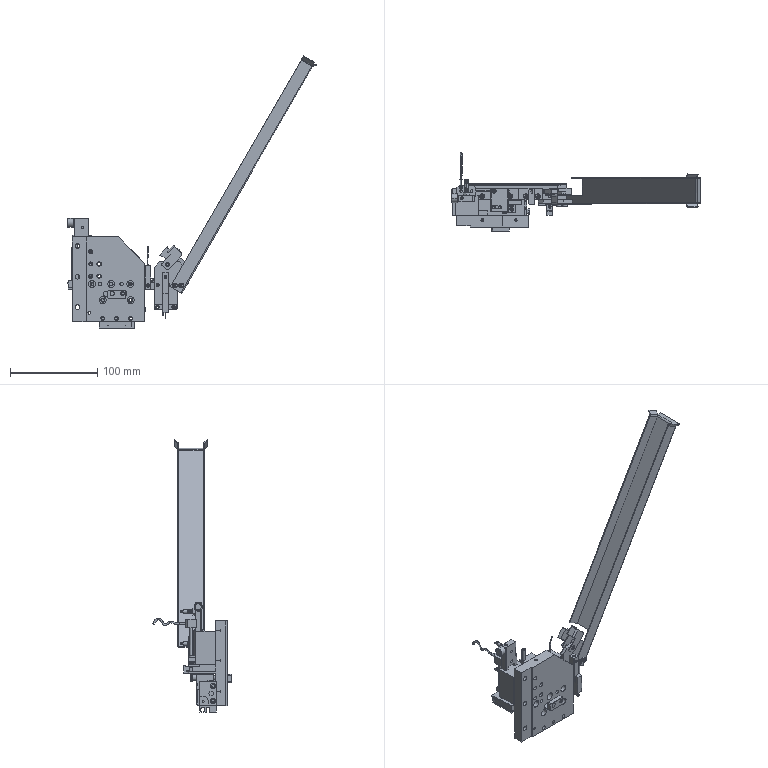Part | NX | 54 solids | 2617 faces | box 286.673 x 90.618 x 312.186 mm | volume 228804 mm3 | plane 1734 | cylinder 596 | cone 255 | spline 18 | torus 13 | sphere 1 | commonest cylinder face diameters 2.5 x110 4 x88 3 x58 3.3 x34 3.5 x30 6 x30